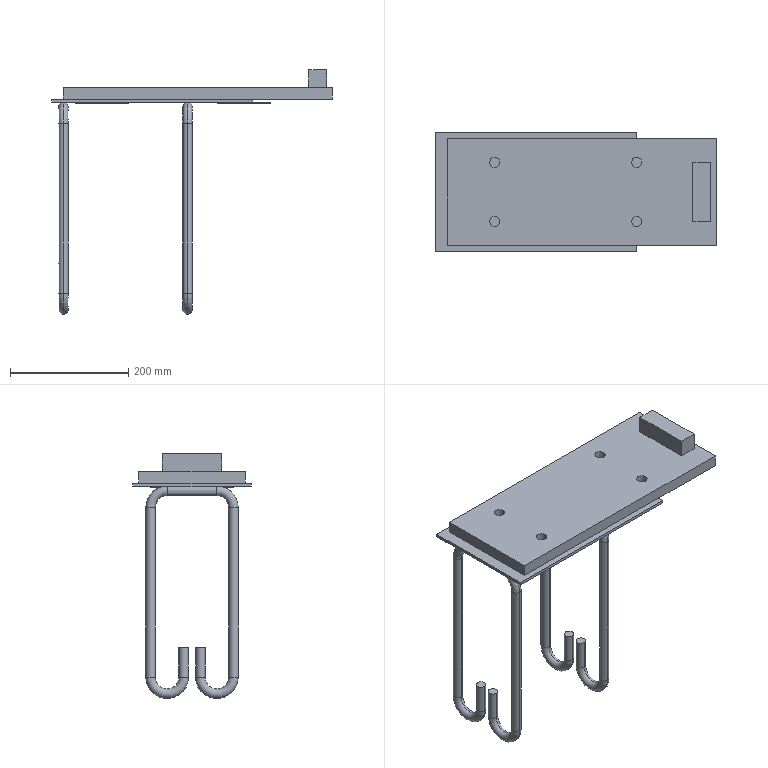Part | SolidWorks | features ICE 3, LPattern 2, Extrusion 1, HoleWzd 1, Sweep 1 | 7 solids | 88 faces | box 475 x 200 x 414 mm | volume 2531678 mm3 | plane 36 | cylinder 36 | torus 16 | commonest cylinder face diameters 16 x20 17.5 x16